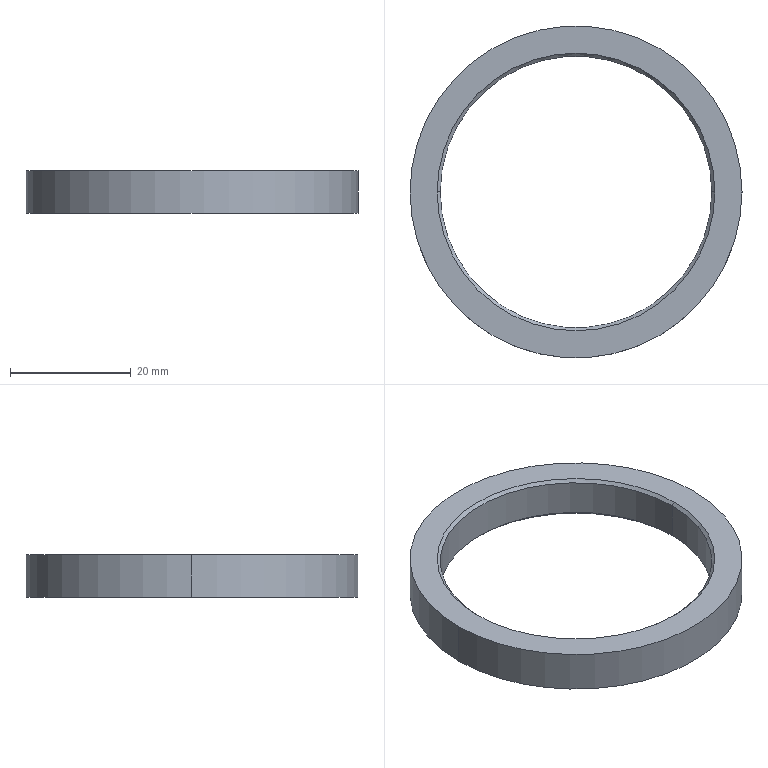Part | SolidWorks | features Revolution 1 | 1 solid | 10 faces | box 55 x 55 x 7 mm | volume 5462 mm3 | cone 4 | cylinder 4 | plane 2 | commonest cylinder face diameters 45 x2 55 x2
STEP:
#1=CARTESIAN_POINT('',(553.731,22.744,-335.193));
#2=VERTEX_POINT('',#1);
#3=CARTESIAN_POINT('',(598.731,22.744,-335.193));
#4=VERTEX_POINT('',#3);
#5=CARTESIAN_POINT('',(576.231,22.744,-335.193));
#6=DIRECTION('',(0.,0.,1.));
#7=DIRECTION('',(1.,0.,0.));
#8=AXIS2_PLACEMENT_3D('',#5,#6,#7);
#9=CIRCLE('',#8,22.5);
#10=EDGE_CURVE('',#2,#4,#9,.T.);
#11=ORIENTED_EDGE('',*,*,#10,.T.);
#12=CARTESIAN_POINT('',(599.231,22.744,-335.693));
#13=VERTEX_POINT('',#12);
#14=CARTESIAN_POINT('',(599.231,22.744,-335.693));
#15=DIRECTION('',(0.7071,0.,-0.7071));
#16=VECTOR('',#15,1000.);
#17=LINE('',#14,#16);
#18=EDGE_CURVE('',#4,#13,#17,.T.);
#19=ORIENTED_EDGE('',*,*,#18,.T.);
#20=CARTESIAN_POINT('',(553.231,22.744,-335.693));
#21=VERTEX_POINT('',#20);
#22=CARTESIAN_POINT('',(576.231,22.744,-335.693));
#23=DIRECTION('',(0.,0.,1.));
#24=DIRECTION('',(1.,0.,0.));
#25=AXIS2_PLACEMENT_3D('',#22,#23,#24);
#26=CIRCLE('',#25,23.);
#27=EDGE_CURVE('',#21,#13,#26,.T.);
#28=ORIENTED_EDGE('',*,*,#27,.F.);
#29=CARTESIAN_POINT('',(553.231,22.744,-335.693));
#30=DIRECTION('',(-0.7071,0.,-0.7071));
#31=VECTOR('',#30,1000.);
#32=LINE('',#29,#31);
#33=EDGE_CURVE('',#2,#21,#32,.T.);
#34=ORIENTED_EDGE('',*,*,#33,.F.);
#35=EDGE_LOOP('',(#11,#19,#28,#34));
#36=FACE_OUTER_BOUND('',#35,.T.);
#37=CARTESIAN_POINT('',(576.231,22.744,-335.693));
#38=DIRECTION('',(0.,0.,-1.));
#39=DIRECTION('',(-1.,0.,0.));
#40=AXIS2_PLACEMENT_3D('',#37,#38,#39);
#41=CONICAL_SURFACE('',#40,23.,0.7854);
#42=ADVANCED_FACE('',(#36),#41,.F.);
#43=CARTESIAN_POINT('',(603.731,22.744,-335.693));
#44=VERTEX_POINT('',#43);
#45=CARTESIAN_POINT('',(548.731,22.744,-335.693));
#46=VERTEX_POINT('',#45);
#47=CARTESIAN_POINT('',(576.231,22.744,-335.693));
#48=DIRECTION('',(0.,0.,1.));
#49=DIRECTION('',(1.,0.,0.));
#50=AXIS2_PLACEMENT_3D('',#47,#48,#49);
#51=CIRCLE('',#50,27.5);
#52=EDGE_CURVE('',#44,#46,#51,.T.);
#53=ORIENTED_EDGE('',*,*,#52,.T.);
#54=CARTESIAN_POINT('',(548.731,22.744,-328.693));
#55=VERTEX_POINT('',#54);
#56=CARTESIAN_POINT('',(548.731,22.744,-335.693));
#57=DIRECTION('',(0.,0.,1.));
#58=VECTOR('',#57,1000.);
#59=LINE('',#56,#58);
#60=EDGE_CURVE('',#46,#55,#59,.T.);
#61=ORIENTED_EDGE('',*,*,#60,.T.);
#62=CARTESIAN_POINT('',(603.731,22.744,-328.693));
#63=VERTEX_POINT('',#62);
#64=CARTESIAN_POINT('',(576.231,22.744,-328.693));
#65=DIRECTION('',(0.,0.,1.));
#66=DIRECTION('',(1.,0.,0.));
#67=AXIS2_PLACEMENT_3D('',#64,#65,#66);
#68=CIRCLE('',#67,27.5);
#69=EDGE_CURVE('',#63,#55,#68,.T.);
#70=ORIENTED_EDGE('',*,*,#69,.F.);
#71=CARTESIAN_POINT('',(603.731,22.744,-335.693));
#72=DIRECTION('',(0.,0.,1.));
#73=VECTOR('',#72,1000.);
#74=LINE('',#71,#73);
#75=EDGE_CURVE('',#44,#63,#74,.T.);
#76=ORIENTED_EDGE('',*,*,#75,.F.);
#77=EDGE_LOOP('',(#53,#61,#70,#76));
#78=FACE_OUTER_BOUND('',#77,.T.);
#79=CARTESIAN_POINT('',(576.231,22.744,-335.693));
#80=DIRECTION('',(0.,0.,1.));
#81=DIRECTION('',(1.,0.,0.));
#82=AXIS2_PLACEMENT_3D('',#79,#80,#81);
#83=CYLINDRICAL_SURFACE('',#82,27.5);
#84=ADVANCED_FACE('',(#78),#83,.T.);
#85=CARTESIAN_POINT('',(553.731,22.744,-329.193));
#86=VERTEX_POINT('',#85);
#87=CARTESIAN_POINT('',(598.731,22.744,-329.193));
#88=VERTEX_POINT('',#87);
#89=CARTESIAN_POINT('',(576.231,22.744,-329.193));
#90=DIRECTION('',(0.,0.,1.));
#91=DIRECTION('',(1.,0.,0.));
#92=AXIS2_PLACEMENT_3D('',#89,#90,#91);
#93=CIRCLE('',#92,22.5);
#94=EDGE_CURVE('',#86,#88,#93,.T.);
#95=ORIENTED_EDGE('',*,*,#94,.F.);
#96=CARTESIAN_POINT('',(553.231,22.744,-328.693));
#97=VERTEX_POINT('',#96);
#98=CARTESIAN_POINT('',(553.731,22.744,-329.193));
#99=DIRECTION('',(-0.7071,0.,0.7071));
#100=VECTOR('',#99,1000.);
#101=LINE('',#98,#100);
#102=EDGE_CURVE('',#86,#97,#101,.T.);
#103=ORIENTED_EDGE('',*,*,#102,.T.);
#104=CARTESIAN_POINT('',(599.231,22.744,-328.693));
#105=VERTEX_POINT('',#104);
#106=CARTESIAN_POINT('',(576.231,22.744,-328.693));
#107=DIRECTION('',(0.,0.,1.));
#108=DIRECTION('',(1.,0.,0.));
#109=AXIS2_PLACEMENT_3D('',#106,#107,#108);
#110=CIRCLE('',#109,23.);
#111=EDGE_CURVE('',#97,#105,#110,.T.);
#112=ORIENTED_EDGE('',*,*,#111,.T.);
#113=CARTESIAN_POINT('',(598.731,22.744,-329.193));
#114=DIRECTION('',(0.7071,0.,0.7071));
#115=VECTOR('',#114,1000.);
#116=LINE('',#113,#115);
#117=EDGE_CURVE('',#88,#105,#116,.T.);
#118=ORIENTED_EDGE('',*,*,#117,.F.);
#119=EDGE_LOOP('',(#95,#103,#112,#118));
#120=FACE_OUTER_BOUND('',#119,.T.);
#121=CARTESIAN_POINT('',(576.231,22.744,-329.193));
#122=DIRECTION('',(0.,0.,1.));
#123=DIRECTION('',(1.,0.,0.));
#124=AXIS2_PLACEMENT_3D('',#121,#122,#123);
#125=CONICAL_SURFACE('',#124,22.5,0.7854);
#126=ADVANCED_FACE('',(#120),#125,.F.);
#127=ORIENTED_EDGE('',*,*,#10,.F.);
#128=CARTESIAN_POINT('',(553.731,22.744,-335.693));
#129=DIRECTION('',(0.,0.,1.));
#130=VECTOR('',#129,1000.);
#131=LINE('',#128,#130);
#132=EDGE_CURVE('',#2,#86,#131,.T.);
#133=ORIENTED_EDGE('',*,*,#132,.T.);
#134=ORIENTED_EDGE('',*,*,#94,.T.);
#135=CARTESIAN_POINT('',(598.731,22.744,-335.693));
#136=DIRECTION('',(0.,0.,1.));
#137=VECTOR('',#136,1000.);
#138=LINE('',#135,#137);
#139=EDGE_CURVE('',#4,#88,#138,.T.);
#140=ORIENTED_EDGE('',*,*,#139,.F.);
#141=EDGE_LOOP('',(#127,#133,#134,#140));
#142=FACE_OUTER_BOUND('',#141,.T.);
#143=CARTESIAN_POINT('',(576.231,22.744,-335.693));
#144=DIRECTION('',(0.,0.,1.));
#145=DIRECTION('',(1.,0.,0.));
#146=AXIS2_PLACEMENT_3D('',#143,#144,#145);
#147=CYLINDRICAL_SURFACE('',#146,22.5);
#148=ADVANCED_FACE('',(#142),#147,.F.);
#149=ORIENTED_EDGE('',*,*,#132,.F.);
#150=CARTESIAN_POINT('',(576.231,22.744,-335.193));
#151=DIRECTION('',(0.,0.,1.));
#152=DIRECTION('',(1.,0.,0.));
#153=AXIS2_PLACEMENT_3D('',#150,#151,#152);
#154=CIRCLE('',#153,22.5);
#155=EDGE_CURVE('',#4,#2,#154,.T.);
#156=ORIENTED_EDGE('',*,*,#155,.F.);
#157=ORIENTED_EDGE('',*,*,#139,.T.);
#158=CARTESIAN_POINT('',(576.231,22.744,-329.193));
#159=DIRECTION('',(0.,0.,1.));
#160=DIRECTION('',(1.,0.,0.));
#161=AXIS2_PLACEMENT_3D('',#158,#159,#160);
#162=CIRCLE('',#161,22.5);
#163=EDGE_CURVE('',#88,#86,#162,.T.);
#164=ORIENTED_EDGE('',*,*,#163,.T.);
#165=EDGE_LOOP('',(#149,#156,#157,#164));
#166=FACE_OUTER_BOUND('',#165,.T.);
#167=CARTESIAN_POINT('',(576.231,22.744,-335.693));
#168=DIRECTION('',(0.,0.,1.));
#169=DIRECTION('',(1.,0.,0.));
#170=AXIS2_PLACEMENT_3D('',#167,#168,#169);
#171=CYLINDRICAL_SURFACE('',#170,22.5);
#172=ADVANCED_FACE('',(#166),#171,.F.);
#173=ORIENTED_EDGE('',*,*,#102,.F.);
#174=ORIENTED_EDGE('',*,*,#163,.F.);
#175=ORIENTED_EDGE('',*,*,#117,.T.);
#176=CARTESIAN_POINT('',(576.231,22.744,-328.693));
#177=DIRECTION('',(0.,0.,1.));
#178=DIRECTION('',(1.,0.,0.));
#179=AXIS2_PLACEMENT_3D('',#176,#177,#178);
#180=CIRCLE('',#179,23.);
#181=EDGE_CURVE('',#105,#97,#180,.T.);
#182=ORIENTED_EDGE('',*,*,#181,.T.);
#183=EDGE_LOOP('',(#173,#174,#175,#182));
#184=FACE_OUTER_BOUND('',#183,.T.);
#185=CARTESIAN_POINT('',(576.231,22.744,-329.193));
#186=DIRECTION('',(0.,0.,1.));
#187=DIRECTION('',(1.,0.,0.));
#188=AXIS2_PLACEMENT_3D('',#185,#186,#187);
#189=CONICAL_SURFACE('',#188,22.5,0.7854);
#190=ADVANCED_FACE('',(#184),#189,.F.);
#191=ORIENTED_EDGE('',*,*,#69,.T.);
#192=CARTESIAN_POINT('',(576.231,22.744,-328.693));
#193=DIRECTION('',(0.,0.,1.));
#194=DIRECTION('',(1.,0.,0.));
#195=AXIS2_PLACEMENT_3D('',#192,#193,#194);
#196=CIRCLE('',#195,27.5);
#197=EDGE_CURVE('',#55,#63,#196,.T.);
#198=ORIENTED_EDGE('',*,*,#197,.T.);
#199=EDGE_LOOP('',(#191,#198));
#200=FACE_OUTER_BOUND('',#199,.T.);
#201=ORIENTED_EDGE('',*,*,#181,.F.);
#202=ORIENTED_EDGE('',*,*,#111,.F.);
#203=EDGE_LOOP('',(#201,#202));
#204=FACE_BOUND('',#203,.T.);
#205=CARTESIAN_POINT('',(599.231,22.744,-328.693));
#206=DIRECTION('',(0.,0.,1.));
#207=DIRECTION('',(1.,0.,0.));
#208=AXIS2_PLACEMENT_3D('',#205,#206,#207);
#209=PLANE('',#208);
#210=ADVANCED_FACE('',(#200,#204),#209,.T.);
#211=ORIENTED_EDGE('',*,*,#60,.F.);
#212=CARTESIAN_POINT('',(576.231,22.744,-335.693));
#213=DIRECTION('',(0.,0.,1.));
#214=DIRECTION('',(1.,0.,0.));
#215=AXIS2_PLACEMENT_3D('',#212,#213,#214);
#216=CIRCLE('',#215,27.5);
#217=EDGE_CURVE('',#46,#44,#216,.T.);
#218=ORIENTED_EDGE('',*,*,#217,.T.);
#219=ORIENTED_EDGE('',*,*,#75,.T.);
#220=ORIENTED_EDGE('',*,*,#197,.F.);
#221=EDGE_LOOP('',(#211,#218,#219,#220));
#222=FACE_OUTER_BOUND('',#221,.T.);
#223=CARTESIAN_POINT('',(576.231,22.744,-335.693));
#224=DIRECTION('',(0.,0.,1.));
#225=DIRECTION('',(1.,0.,0.));
#226=AXIS2_PLACEMENT_3D('',#223,#224,#225);
#227=CYLINDRICAL_SURFACE('',#226,27.5);
#228=ADVANCED_FACE('',(#222),#227,.T.);
#229=ORIENTED_EDGE('',*,*,#27,.T.);
#230=CARTESIAN_POINT('',(576.231,22.744,-335.693));
#231=DIRECTION('',(0.,0.,1.));
#232=DIRECTION('',(1.,0.,0.));
#233=AXIS2_PLACEMENT_3D('',#230,#231,#232);
#234=CIRCLE('',#233,23.);
#235=EDGE_CURVE('',#13,#21,#234,.T.);
#236=ORIENTED_EDGE('',*,*,#235,.T.);
#237=EDGE_LOOP('',(#229,#236));
#238=FACE_BOUND('',#237,.T.);
#239=ORIENTED_EDGE('',*,*,#52,.F.);
#240=ORIENTED_EDGE('',*,*,#217,.F.);
#241=EDGE_LOOP('',(#239,#240));
#242=FACE_OUTER_BOUND('',#241,.T.);
#243=CARTESIAN_POINT('',(603.731,22.744,-335.693));
#244=DIRECTION('',(0.,0.,-1.));
#245=DIRECTION('',(-1.,0.,0.));
#246=AXIS2_PLACEMENT_3D('',#243,#244,#245);
#247=PLANE('',#246);
#248=ADVANCED_FACE('',(#238,#242),#247,.T.);
#249=ORIENTED_EDGE('',*,*,#18,.F.);
#250=ORIENTED_EDGE('',*,*,#155,.T.);
#251=ORIENTED_EDGE('',*,*,#33,.T.);
#252=ORIENTED_EDGE('',*,*,#235,.F.);
#253=EDGE_LOOP('',(#249,#250,#251,#252));
#254=FACE_OUTER_BOUND('',#253,.T.);
#255=CARTESIAN_POINT('',(576.231,22.744,-335.693));
#256=DIRECTION('',(0.,0.,-1.));
#257=DIRECTION('',(-1.,0.,0.));
#258=AXIS2_PLACEMENT_3D('',#255,#256,#257);
#259=CONICAL_SURFACE('',#258,23.,0.7854);
#260=ADVANCED_FACE('',(#254),#259,.F.);
#261=CLOSED_SHELL('',(#42,#84,#126,#148,#172,#190,#210,#228,#248,#260));
#262=MANIFOLD_SOLID_BREP('',#261);
#263=CARTESIAN_POINT('',(0.,0.,0.));
#264=DIRECTION('',(0.,0.,1.));
#265=DIRECTION('',(1.,0.,0.));
#266=AXIS2_PLACEMENT_3D('',#263,#264,#265);
#267=(LENGTH_UNIT()NAMED_UNIT(*)SI_UNIT(.MILLI.,.METRE.));
#268=UNCERTAINTY_MEASURE_WITH_UNIT(LENGTH_MEASURE(0.00001),#267,'','');
#269=(NAMED_UNIT(*)PLANE_ANGLE_UNIT()SI_UNIT($,.RADIAN.));
#270=(NAMED_UNIT(*)SI_UNIT($,.STERADIAN.)SOLID_ANGLE_UNIT());
#271=(GEOMETRIC_REPRESENTATION_CONTEXT(3)GLOBAL_UNCERTAINTY_ASSIGNED_CONTEXT((#268))GLOBAL_UNIT_ASSIGNED_CONTEXT((#267,#269,#270))REPRESENTATION_CONTEXT('',''));
#272=ADVANCED_BREP_SHAPE_REPRESENTATION('',(#262,#266),#271);